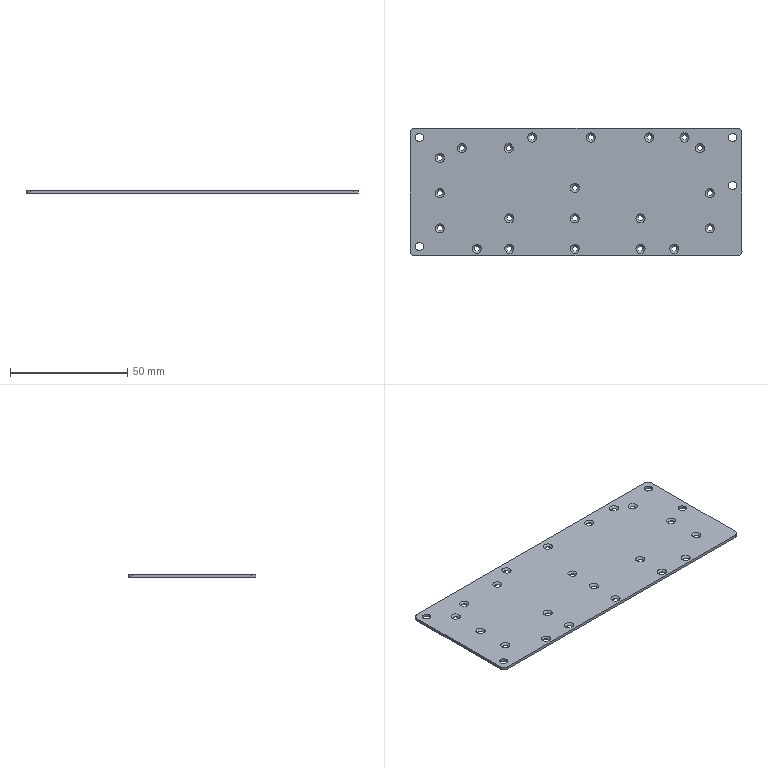Part | STEP file | 1 to 8 power divider cover | 1 solid | 77 faces | box 141.709 x 54.52 x 1.2 mm | volume 9052 mm3 | cone 42 | cylinder 29 | plane 6 | commonest cylinder face diameters 2.2 x21 3.5 x4 4 x4